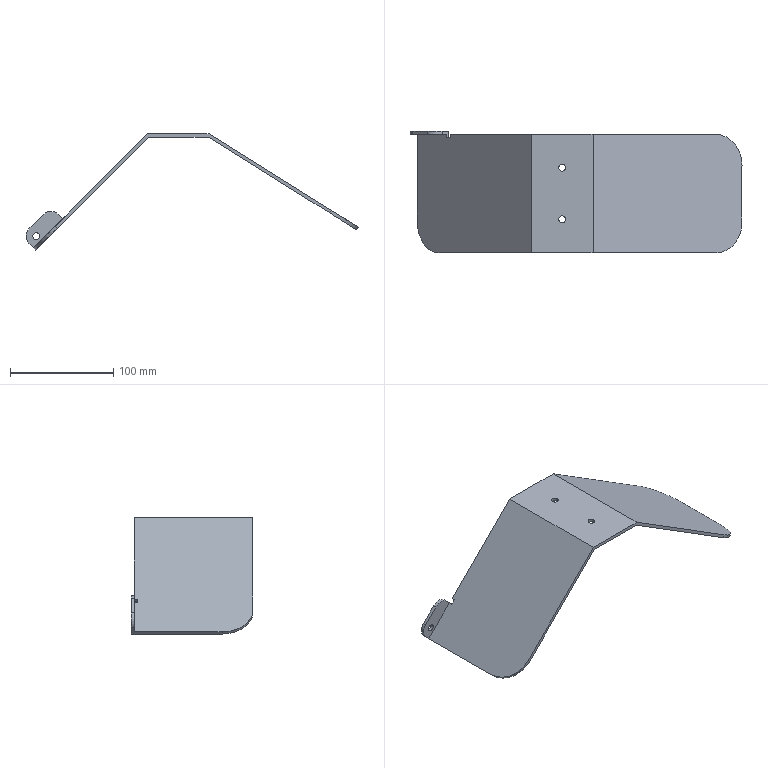Part | SolidWorks | features BaseBody 1 | 1 solid | 27 faces | box 321.953 x 118.25 x 112.625 mm | volume 132694 mm3 | plane 16 | cylinder 11 | commonest cylinder face diameters 6.5 x6 60 x3 20 x2
STEP:
#1=CARTESIAN_POINT('',(617.2,21.,201.536));
#2=VERTEX_POINT('',#1);
#3=CARTESIAN_POINT('',(623.7,21.,201.536));
#4=VERTEX_POINT('',#3);
#5=CARTESIAN_POINT('',(620.45,21.,201.536));
#6=DIRECTION('',(0.,0.,-1.));
#7=DIRECTION('',(1.,0.,0.));
#8=AXIS2_PLACEMENT_3D('',#5,#6,#7);
#9=CIRCLE('',#8,3.25);
#10=EDGE_CURVE('',#2,#4,#9,.T.);
#11=ORIENTED_EDGE('',*,*,#10,.F.);
#12=CARTESIAN_POINT('',(617.2,21.,198.536));
#13=VERTEX_POINT('',#12);
#14=CARTESIAN_POINT('',(617.2,21.,230.536));
#15=DIRECTION('',(0.,0.,-1.));
#16=VECTOR('',#15,1000.);
#17=LINE('',#14,#16);
#18=EDGE_CURVE('',#2,#13,#17,.T.);
#19=ORIENTED_EDGE('',*,*,#18,.T.);
#20=CARTESIAN_POINT('',(623.7,21.,198.536));
#21=VERTEX_POINT('',#20);
#22=CARTESIAN_POINT('',(620.45,21.,198.536));
#23=DIRECTION('',(0.,0.,1.));
#24=DIRECTION('',(1.,0.,0.));
#25=AXIS2_PLACEMENT_3D('',#22,#23,#24);
#26=CIRCLE('',#25,3.25);
#27=EDGE_CURVE('',#21,#13,#26,.T.);
#28=ORIENTED_EDGE('',*,*,#27,.F.);
#29=CARTESIAN_POINT('',(623.7,21.,230.536));
#30=DIRECTION('',(0.,0.,-1.));
#31=VECTOR('',#30,1000.);
#32=LINE('',#29,#31);
#33=EDGE_CURVE('',#4,#21,#32,.T.);
#34=ORIENTED_EDGE('',*,*,#33,.F.);
#35=EDGE_LOOP('',(#11,#19,#28,#34));
#36=FACE_OUTER_BOUND('',#35,.T.);
#37=CARTESIAN_POINT('',(620.45,21.,230.536));
#38=DIRECTION('',(0.,0.,-1.));
#39=DIRECTION('',(1.,0.,0.));
#40=AXIS2_PLACEMENT_3D('',#37,#38,#39);
#41=CYLINDRICAL_SURFACE('',#40,3.25);
#42=ADVANCED_FACE('',(#36),#41,.F.);
#43=CARTESIAN_POINT('',(617.2,-29.,201.536));
#44=VERTEX_POINT('',#43);
#45=CARTESIAN_POINT('',(623.7,-29.,201.536));
#46=VERTEX_POINT('',#45);
#47=CARTESIAN_POINT('',(620.45,-29.,201.536));
#48=DIRECTION('',(0.,0.,-1.));
#49=DIRECTION('',(1.,0.,0.));
#50=AXIS2_PLACEMENT_3D('',#47,#48,#49);
#51=CIRCLE('',#50,3.25);
#52=EDGE_CURVE('',#44,#46,#51,.T.);
#53=ORIENTED_EDGE('',*,*,#52,.F.);
#54=CARTESIAN_POINT('',(617.2,-29.,198.536));
#55=VERTEX_POINT('',#54);
#56=CARTESIAN_POINT('',(617.2,-29.,230.536));
#57=DIRECTION('',(0.,0.,-1.));
#58=VECTOR('',#57,1000.);
#59=LINE('',#56,#58);
#60=EDGE_CURVE('',#44,#55,#59,.T.);
#61=ORIENTED_EDGE('',*,*,#60,.T.);
#62=CARTESIAN_POINT('',(623.7,-29.,198.536));
#63=VERTEX_POINT('',#62);
#64=CARTESIAN_POINT('',(620.45,-29.,198.536));
#65=DIRECTION('',(0.,0.,1.));
#66=DIRECTION('',(1.,0.,0.));
#67=AXIS2_PLACEMENT_3D('',#64,#65,#66);
#68=CIRCLE('',#67,3.25);
#69=EDGE_CURVE('',#63,#55,#68,.T.);
#70=ORIENTED_EDGE('',*,*,#69,.F.);
#71=CARTESIAN_POINT('',(623.7,-29.,230.536));
#72=DIRECTION('',(0.,0.,-1.));
#73=VECTOR('',#72,1000.);
#74=LINE('',#71,#73);
#75=EDGE_CURVE('',#46,#63,#74,.T.);
#76=ORIENTED_EDGE('',*,*,#75,.F.);
#77=EDGE_LOOP('',(#53,#61,#70,#76));
#78=FACE_OUTER_BOUND('',#77,.T.);
#79=CARTESIAN_POINT('',(620.45,-29.,230.536));
#80=DIRECTION('',(0.,0.,-1.));
#81=DIRECTION('',(1.,0.,0.));
#82=AXIS2_PLACEMENT_3D('',#79,#80,#81);
#83=CYLINDRICAL_SURFACE('',#82,3.25);
#84=ADVANCED_FACE('',(#78),#83,.F.);
#85=CARTESIAN_POINT('',(486.098,56.75,102.629));
#86=VERTEX_POINT('',#85);
#87=CARTESIAN_POINT('',(479.623,56.75,102.063));
#88=VERTEX_POINT('',#87);
#89=CARTESIAN_POINT('',(482.86,56.75,102.346));
#90=DIRECTION('',(0.,-1.,0.));
#91=DIRECTION('',(0.,0.,1.));
#92=AXIS2_PLACEMENT_3D('',#89,#90,#91);
#93=CIRCLE('',#92,3.25);
#94=EDGE_CURVE('',#86,#88,#93,.T.);
#95=ORIENTED_EDGE('',*,*,#94,.F.);
#96=CARTESIAN_POINT('',(486.098,53.75,102.629));
#97=VERTEX_POINT('',#96);
#98=CARTESIAN_POINT('',(486.098,94.,102.629));
#99=DIRECTION('',(0.,-1.,0.));
#100=VECTOR('',#99,1000.);
#101=LINE('',#98,#100);
#102=EDGE_CURVE('',#86,#97,#101,.T.);
#103=ORIENTED_EDGE('',*,*,#102,.T.);
#104=CARTESIAN_POINT('',(479.623,53.75,102.063));
#105=VERTEX_POINT('',#104);
#106=CARTESIAN_POINT('',(482.86,53.75,102.346));
#107=DIRECTION('',(0.,1.,0.));
#108=DIRECTION('',(0.,0.,1.));
#109=AXIS2_PLACEMENT_3D('',#106,#107,#108);
#110=CIRCLE('',#109,3.25);
#111=EDGE_CURVE('',#105,#97,#110,.T.);
#112=ORIENTED_EDGE('',*,*,#111,.F.);
#113=CARTESIAN_POINT('',(479.623,94.,102.063));
#114=DIRECTION('',(0.,-1.,0.));
#115=VECTOR('',#114,1000.);
#116=LINE('',#113,#115);
#117=EDGE_CURVE('',#88,#105,#116,.T.);
#118=ORIENTED_EDGE('',*,*,#117,.F.);
#119=EDGE_LOOP('',(#95,#103,#112,#118));
#120=FACE_OUTER_BOUND('',#119,.T.);
#121=CARTESIAN_POINT('',(482.86,94.,102.346));
#122=DIRECTION('',(0.,-1.,0.));
#123=DIRECTION('',(-0.9962,0.,-0.08716));
#124=AXIS2_PLACEMENT_3D('',#121,#122,#123);
#125=CYLINDRICAL_SURFACE('',#124,3.25);
#126=ADVANCED_FACE('',(#120),#125,.F.);
#127=CARTESIAN_POINT('',(511.852,50.5,122.852));
#128=VERTEX_POINT('',#127);
#129=CARTESIAN_POINT('',(511.852,53.5,122.852));
#130=VERTEX_POINT('',#129);
#131=CARTESIAN_POINT('',(511.852,-4.,122.852));
#132=DIRECTION('',(0.,1.,0.));
#133=VECTOR('',#132,1000.);
#134=LINE('',#131,#133);
#135=EDGE_CURVE('',#128,#130,#134,.T.);
#136=ORIENTED_EDGE('',*,*,#135,.T.);
#137=CARTESIAN_POINT('',(513.973,53.5,120.731));
#138=VERTEX_POINT('',#137);
#139=CARTESIAN_POINT('',(511.852,53.5,122.852));
#140=DIRECTION('',(0.7071,0.,-0.7071));
#141=VECTOR('',#140,1000.);
#142=LINE('',#139,#141);
#143=EDGE_CURVE('',#130,#138,#142,.T.);
#144=ORIENTED_EDGE('',*,*,#143,.T.);
#145=CARTESIAN_POINT('',(513.973,50.5,120.731));
#146=VERTEX_POINT('',#145);
#147=CARTESIAN_POINT('',(513.973,-4.,120.731));
#148=DIRECTION('',(0.,1.,0.));
#149=VECTOR('',#148,1000.);
#150=LINE('',#147,#149);
#151=EDGE_CURVE('',#146,#138,#150,.T.);
#152=ORIENTED_EDGE('',*,*,#151,.F.);
#153=CARTESIAN_POINT('',(500.538,50.5,134.166));
#154=DIRECTION('',(0.7071,0.,-0.7071));
#155=VECTOR('',#154,1000.);
#156=LINE('',#153,#155);
#157=EDGE_CURVE('',#128,#146,#156,.T.);
#158=ORIENTED_EDGE('',*,*,#157,.F.);
#159=EDGE_LOOP('',(#136,#144,#152,#158));
#160=FACE_OUTER_BOUND('',#159,.T.);
#161=CARTESIAN_POINT('',(511.852,57.,122.852));
#162=DIRECTION('',(-0.7071,0.,-0.7071));
#163=DIRECTION('',(-0.7071,0.,0.7071));
#164=AXIS2_PLACEMENT_3D('',#161,#162,#163);
#165=PLANE('',#164);
#166=ADVANCED_FACE('',(#160),#165,.T.);
#167=ORIENTED_EDGE('',*,*,#157,.T.);
#168=CARTESIAN_POINT('',(510.437,50.5,117.195));
#169=VERTEX_POINT('',#168);
#170=CARTESIAN_POINT('',(596.251,50.5,203.009));
#171=DIRECTION('',(-0.7071,0.,-0.7071));
#172=VECTOR('',#171,1000.);
#173=LINE('',#170,#172);
#174=EDGE_CURVE('',#146,#169,#173,.T.);
#175=ORIENTED_EDGE('',*,*,#174,.T.);
#176=CARTESIAN_POINT('',(508.316,50.5,119.316));
#177=VERTEX_POINT('',#176);
#178=CARTESIAN_POINT('',(508.316,50.5,119.316));
#179=DIRECTION('',(-0.7071,0.,0.7071));
#180=VECTOR('',#179,1000.);
#181=LINE('',#178,#180);
#182=EDGE_CURVE('',#169,#177,#181,.T.);
#183=ORIENTED_EDGE('',*,*,#182,.T.);
#184=CARTESIAN_POINT('',(594.13,50.5,205.13));
#185=DIRECTION('',(-0.7071,0.,-0.7071));
#186=VECTOR('',#185,1000.);
#187=LINE('',#184,#186);
#188=EDGE_CURVE('',#128,#177,#187,.T.);
#189=ORIENTED_EDGE('',*,*,#188,.F.);
#190=EDGE_LOOP('',(#167,#175,#183,#189));
#191=FACE_OUTER_BOUND('',#190,.T.);
#192=CARTESIAN_POINT('',(500.538,50.5,134.166));
#193=DIRECTION('',(0.,-1.,0.));
#194=DIRECTION('',(0.,0.,-1.));
#195=AXIS2_PLACEMENT_3D('',#192,#193,#194);
#196=PLANE('',#195);
#197=ADVANCED_FACE('',(#191),#196,.F.);
#198=CARTESIAN_POINT('',(767.782,53.5,124.627));
#199=VERTEX_POINT('',#198);
#200=CARTESIAN_POINT('',(793.223,23.5,108.73));
#201=VERTEX_POINT('',#200);
#202=CARTESIAN_POINT('',(767.782,23.5,124.627));
#203=DIRECTION('',(-0.5299,0.,-0.848));
#204=DIRECTION('',(-0.848,0.,0.5299));
#205=AXIS2_PLACEMENT_3D('',#202,#203,#204);
#206=CIRCLE('',#205,30.);
#207=EDGE_CURVE('',#199,#201,#206,.T.);
#208=ORIENTED_EDGE('',*,*,#207,.T.);
#209=CARTESIAN_POINT('',(793.223,-31.5,108.73));
#210=VERTEX_POINT('',#209);
#211=CARTESIAN_POINT('',(793.223,46.,108.73));
#212=DIRECTION('',(0.,-1.,0.));
#213=VECTOR('',#212,1000.);
#214=LINE('',#211,#213);
#215=EDGE_CURVE('',#201,#210,#214,.T.);
#216=ORIENTED_EDGE('',*,*,#215,.T.);
#217=CARTESIAN_POINT('',(767.782,-61.5,124.627));
#218=VERTEX_POINT('',#217);
#219=CARTESIAN_POINT('',(767.782,-31.5,124.627));
#220=DIRECTION('',(-0.5299,0.,-0.848));
#221=DIRECTION('',(0.848,0.,-0.5299));
#222=AXIS2_PLACEMENT_3D('',#219,#220,#221);
#223=CIRCLE('',#222,30.);
#224=EDGE_CURVE('',#210,#218,#223,.T.);
#225=ORIENTED_EDGE('',*,*,#224,.T.);
#226=CARTESIAN_POINT('',(649.504,-61.5,198.536));
#227=VERTEX_POINT('',#226);
#228=CARTESIAN_POINT('',(616.757,-61.5,218.998));
#229=DIRECTION('',(0.848,0.,-0.5299));
#230=VECTOR('',#229,1000.);
#231=LINE('',#228,#230);
#232=EDGE_CURVE('',#227,#218,#231,.T.);
#233=ORIENTED_EDGE('',*,*,#232,.F.);
#234=CARTESIAN_POINT('',(649.504,53.5,198.536));
#235=VERTEX_POINT('',#234);
#236=CARTESIAN_POINT('',(649.504,-4.,198.536));
#237=DIRECTION('',(0.,1.,0.));
#238=VECTOR('',#237,1000.);
#239=LINE('',#236,#238);
#240=EDGE_CURVE('',#227,#235,#239,.T.);
#241=ORIENTED_EDGE('',*,*,#240,.T.);
#242=CARTESIAN_POINT('',(624.235,53.5,214.325));
#243=DIRECTION('',(-0.848,0.,0.5299));
#244=VECTOR('',#243,1000.);
#245=LINE('',#242,#244);
#246=EDGE_CURVE('',#199,#235,#245,.T.);
#247=ORIENTED_EDGE('',*,*,#246,.F.);
#248=EDGE_LOOP('',(#208,#216,#225,#233,#241,#247));
#249=FACE_OUTER_BOUND('',#248,.T.);
#250=CARTESIAN_POINT('',(616.757,-4.,218.998));
#251=DIRECTION('',(-0.5299,0.,-0.848));
#252=DIRECTION('',(-0.848,0.,0.5299));
#253=AXIS2_PLACEMENT_3D('',#250,#251,#252);
#254=PLANE('',#253);
#255=ADVANCED_FACE('',(#249),#254,.T.);
#256=CARTESIAN_POINT('',(769.372,-61.5,127.172));
#257=VERTEX_POINT('',#256);
#258=CARTESIAN_POINT('',(767.782,-61.5,124.627));
#259=DIRECTION('',(0.5299,0.,0.848));
#260=VECTOR('',#259,1000.);
#261=LINE('',#258,#260);
#262=EDGE_CURVE('',#218,#257,#261,.T.);
#263=ORIENTED_EDGE('',*,*,#262,.F.);
#264=ORIENTED_EDGE('',*,*,#224,.F.);
#265=CARTESIAN_POINT('',(794.813,-31.5,111.274));
#266=VERTEX_POINT('',#265);
#267=CARTESIAN_POINT('',(793.223,-31.5,108.73));
#268=DIRECTION('',(0.5299,0.,0.848));
#269=VECTOR('',#268,1000.);
#270=LINE('',#267,#269);
#271=EDGE_CURVE('',#210,#266,#270,.T.);
#272=ORIENTED_EDGE('',*,*,#271,.T.);
#273=CARTESIAN_POINT('',(769.372,-31.5,127.172));
#274=DIRECTION('',(0.5299,0.,0.848));
#275=DIRECTION('',(0.,-1.,0.));
#276=AXIS2_PLACEMENT_3D('',#273,#274,#275);
#277=CIRCLE('',#276,30.);
#278=EDGE_CURVE('',#257,#266,#277,.T.);
#279=ORIENTED_EDGE('',*,*,#278,.F.);
#280=EDGE_LOOP('',(#263,#264,#272,#279));
#281=FACE_OUTER_BOUND('',#280,.T.);
#282=CARTESIAN_POINT('',(769.372,-31.5,127.172));
#283=DIRECTION('',(-0.5299,0.,-0.848));
#284=DIRECTION('',(-0.848,0.,0.5299));
#285=AXIS2_PLACEMENT_3D('',#282,#283,#284);
#286=CYLINDRICAL_SURFACE('',#285,30.);
#287=ADVANCED_FACE('',(#281),#286,.T.);
#288=CARTESIAN_POINT('',(794.813,23.5,111.274));
#289=VERTEX_POINT('',#288);
#290=CARTESIAN_POINT('',(794.813,23.5,111.274));
#291=DIRECTION('',(-0.5299,0.,-0.848));
#292=VECTOR('',#291,1000.);
#293=LINE('',#290,#292);
#294=EDGE_CURVE('',#289,#201,#293,.T.);
#295=ORIENTED_EDGE('',*,*,#294,.T.);
#296=ORIENTED_EDGE('',*,*,#207,.F.);
#297=CARTESIAN_POINT('',(769.372,53.5,127.172));
#298=VERTEX_POINT('',#297);
#299=CARTESIAN_POINT('',(769.372,53.5,127.172));
#300=DIRECTION('',(-0.5299,0.,-0.848));
#301=VECTOR('',#300,1000.);
#302=LINE('',#299,#301);
#303=EDGE_CURVE('',#298,#199,#302,.T.);
#304=ORIENTED_EDGE('',*,*,#303,.F.);
#305=CARTESIAN_POINT('',(769.372,23.5,127.172));
#306=DIRECTION('',(0.5299,0.,0.848));
#307=DIRECTION('',(-0.848,0.,0.5299));
#308=AXIS2_PLACEMENT_3D('',#305,#306,#307);
#309=CIRCLE('',#308,30.);
#310=EDGE_CURVE('',#289,#298,#309,.T.);
#311=ORIENTED_EDGE('',*,*,#310,.F.);
#312=EDGE_LOOP('',(#295,#296,#304,#311));
#313=FACE_OUTER_BOUND('',#312,.T.);
#314=CARTESIAN_POINT('',(769.372,23.5,127.172));
#315=DIRECTION('',(-0.5299,0.,-0.848));
#316=DIRECTION('',(0.848,0.,-0.5299));
#317=AXIS2_PLACEMENT_3D('',#314,#315,#316);
#318=CYLINDRICAL_SURFACE('',#317,30.);
#319=ADVANCED_FACE('',(#313),#318,.T.);
#320=ORIENTED_EDGE('',*,*,#294,.F.);
#321=CARTESIAN_POINT('',(794.813,46.,111.274));
#322=DIRECTION('',(0.,-1.,0.));
#323=VECTOR('',#322,1000.);
#324=LINE('',#321,#323);
#325=EDGE_CURVE('',#289,#266,#324,.T.);
#326=ORIENTED_EDGE('',*,*,#325,.T.);
#327=ORIENTED_EDGE('',*,*,#271,.F.);
#328=ORIENTED_EDGE('',*,*,#215,.F.);
#329=EDGE_LOOP('',(#320,#326,#327,#328));
#330=FACE_OUTER_BOUND('',#329,.T.);
#331=CARTESIAN_POINT('',(794.813,46.,111.274));
#332=DIRECTION('',(-0.848,0.,0.5299));
#333=DIRECTION('',(0.,1.,0.));
#334=AXIS2_PLACEMENT_3D('',#331,#332,#333);
#335=PLANE('',#334);
#336=ADVANCED_FACE('',(#330),#335,.F.);
#337=CARTESIAN_POINT('',(650.364,-61.5,201.536));
#338=VERTEX_POINT('',#337);
#339=CARTESIAN_POINT('',(650.364,53.5,201.536));
#340=VERTEX_POINT('',#339);
#341=CARTESIAN_POINT('',(650.364,-4.,201.536));
#342=DIRECTION('',(0.,1.,0.));
#343=VECTOR('',#342,1000.);
#344=LINE('',#341,#343);
#345=EDGE_CURVE('',#338,#340,#344,.T.);
#346=ORIENTED_EDGE('',*,*,#345,.F.);
#347=CARTESIAN_POINT('',(618.347,-61.5,221.542));
#348=DIRECTION('',(-0.848,0.,0.5299));
#349=VECTOR('',#348,1000.);
#350=LINE('',#347,#349);
#351=EDGE_CURVE('',#257,#338,#350,.T.);
#352=ORIENTED_EDGE('',*,*,#351,.F.);
#353=ORIENTED_EDGE('',*,*,#278,.T.);
#354=ORIENTED_EDGE('',*,*,#325,.F.);
#355=ORIENTED_EDGE('',*,*,#310,.T.);
#356=CARTESIAN_POINT('',(618.347,53.5,221.542));
#357=DIRECTION('',(-0.848,0.,0.5299));
#358=VECTOR('',#357,1000.);
#359=LINE('',#356,#358);
#360=EDGE_CURVE('',#298,#340,#359,.T.);
#361=ORIENTED_EDGE('',*,*,#360,.T.);
#362=EDGE_LOOP('',(#346,#352,#353,#354,#355,#361));
#363=FACE_OUTER_BOUND('',#362,.T.);
#364=CARTESIAN_POINT('',(618.347,-4.,221.542));
#365=DIRECTION('',(-0.5299,0.,-0.848));
#366=DIRECTION('',(-0.848,0.,0.5299));
#367=AXIS2_PLACEMENT_3D('',#364,#365,#366);
#368=PLANE('',#367);
#369=ADVANCED_FACE('',(#363),#368,.F.);
#370=CARTESIAN_POINT('',(482.153,56.75,88.911));
#371=VERTEX_POINT('',#370);
#372=CARTESIAN_POINT('',(475.789,56.75,95.275));
#373=VERTEX_POINT('',#372);
#374=CARTESIAN_POINT('',(480.032,56.75,91.032));
#375=DIRECTION('',(-0.7071,0.,0.7071));
#376=VECTOR('',#375,1000.);
#377=LINE('',#374,#376);
#378=EDGE_CURVE('',#371,#373,#377,.T.);
#379=ORIENTED_EDGE('',*,*,#378,.F.);
#380=CARTESIAN_POINT('',(482.153,-31.5,88.911));
#381=VERTEX_POINT('',#380);
#382=CARTESIAN_POINT('',(482.153,-24.,88.911));
#383=DIRECTION('',(0.,1.,0.));
#384=VECTOR('',#383,1000.);
#385=LINE('',#382,#384);
#386=EDGE_CURVE('',#381,#371,#385,.T.);
#387=ORIENTED_EDGE('',*,*,#386,.F.);
#388=CARTESIAN_POINT('',(480.032,-31.5,91.032));
#389=VERTEX_POINT('',#388);
#390=CARTESIAN_POINT('',(480.032,-31.5,91.032));
#391=DIRECTION('',(0.7071,0.,-0.7071));
#392=VECTOR('',#391,1000.);
#393=LINE('',#390,#392);
#394=EDGE_CURVE('',#389,#381,#393,.T.);
#395=ORIENTED_EDGE('',*,*,#394,.F.);
#396=CARTESIAN_POINT('',(480.032,53.75,91.032));
#397=VERTEX_POINT('',#396);
#398=CARTESIAN_POINT('',(480.032,-24.,91.032));
#399=DIRECTION('',(0.,1.,0.));
#400=VECTOR('',#399,1000.);
#401=LINE('',#398,#400);
#402=EDGE_CURVE('',#389,#397,#401,.T.);
#403=ORIENTED_EDGE('',*,*,#402,.T.);
#404=CARTESIAN_POINT('',(475.789,53.75,95.275));
#405=VERTEX_POINT('',#404);
#406=CARTESIAN_POINT('',(468.718,53.75,102.346));
#407=DIRECTION('',(0.7071,0.,-0.7071));
#408=VECTOR('',#407,1000.);
#409=LINE('',#406,#408);
#410=EDGE_CURVE('',#405,#397,#409,.T.);
#411=ORIENTED_EDGE('',*,*,#410,.F.);
#412=CARTESIAN_POINT('',(475.789,57.,95.275));
#413=DIRECTION('',(0.,-1.,0.));
#414=VECTOR('',#413,1000.);
#415=LINE('',#412,#414);
#416=EDGE_CURVE('',#373,#405,#415,.T.);
#417=ORIENTED_EDGE('',*,*,#416,.F.);
#418=EDGE_LOOP('',(#379,#387,#395,#403,#411,#417));
#419=FACE_OUTER_BOUND('',#418,.T.);
#420=CARTESIAN_POINT('',(480.032,-54.,91.032));
#421=DIRECTION('',(0.7071,0.,0.7071));
#422=DIRECTION('',(0.,-1.,0.));
#423=AXIS2_PLACEMENT_3D('',#420,#421,#422);
#424=PLANE('',#423);
#425=ADVANCED_FACE('',(#419),#424,.F.);
#426=ORIENTED_EDGE('',*,*,#111,.T.);
#427=CARTESIAN_POINT('',(482.86,53.75,102.346));
#428=DIRECTION('',(0.,1.,0.));
#429=DIRECTION('',(0.,0.,1.));
#430=AXIS2_PLACEMENT_3D('',#427,#428,#429);
#431=CIRCLE('',#430,3.25);
#432=EDGE_CURVE('',#97,#105,#431,.T.);
#433=ORIENTED_EDGE('',*,*,#432,.T.);
#434=EDGE_LOOP('',(#426,#433));
#435=FACE_BOUND('',#434,.T.);
#436=ORIENTED_EDGE('',*,*,#410,.T.);
#437=CARTESIAN_POINT('',(508.316,53.75,119.316));
#438=VERTEX_POINT('',#437);
#439=CARTESIAN_POINT('',(594.13,53.75,205.13));
#440=DIRECTION('',(0.7071,0.,0.7071));
#441=VECTOR('',#440,1000.);
#442=LINE('',#439,#441);
#443=EDGE_CURVE('',#397,#438,#442,.T.);
#444=ORIENTED_EDGE('',*,*,#443,.T.);
#445=CARTESIAN_POINT('',(504.073,53.75,123.559));
#446=VERTEX_POINT('',#445);
#447=CARTESIAN_POINT('',(497.002,53.75,130.63));
#448=DIRECTION('',(-0.7071,0.,0.7071));
#449=VECTOR('',#448,1000.);
#450=LINE('',#447,#449);
#451=EDGE_CURVE('',#438,#446,#450,.T.);
#452=ORIENTED_EDGE('',*,*,#451,.T.);
#453=CARTESIAN_POINT('',(489.931,53.75,123.559));
#454=VERTEX_POINT('',#453);
#455=CARTESIAN_POINT('',(497.002,53.75,116.488));
#456=DIRECTION('',(0.,-1.,0.));
#457=DIRECTION('',(0.,0.,1.));
#458=AXIS2_PLACEMENT_3D('',#455,#456,#457);
#459=CIRCLE('',#458,10.);
#460=EDGE_CURVE('',#446,#454,#459,.T.);
#461=ORIENTED_EDGE('',*,*,#460,.T.);
#462=CARTESIAN_POINT('',(475.789,53.75,109.417));
#463=VERTEX_POINT('',#462);
#464=CARTESIAN_POINT('',(582.816,53.75,216.444));
#465=DIRECTION('',(-0.7071,0.,-0.7071));
#466=VECTOR('',#465,1000.);
#467=LINE('',#464,#466);
#468=EDGE_CURVE('',#454,#463,#467,.T.);
#469=ORIENTED_EDGE('',*,*,#468,.T.);
#470=CARTESIAN_POINT('',(482.86,53.75,102.346));
#471=DIRECTION('',(0.,-1.,0.));
#472=DIRECTION('',(0.,0.,1.));
#473=AXIS2_PLACEMENT_3D('',#470,#471,#472);
#474=CIRCLE('',#473,10.);
#475=EDGE_CURVE('',#463,#405,#474,.T.);
#476=ORIENTED_EDGE('',*,*,#475,.T.);
#477=EDGE_LOOP('',(#436,#444,#452,#461,#469,#476));
#478=FACE_OUTER_BOUND('',#477,.T.);
#479=CARTESIAN_POINT('',(468.718,53.75,102.346));
#480=DIRECTION('',(0.,1.,0.));
#481=DIRECTION('',(1.,0.,0.));
#482=AXIS2_PLACEMENT_3D('',#479,#480,#481);
#483=PLANE('',#482);
#484=ADVANCED_FACE('',(#435,#478),#483,.F.);
#485=CARTESIAN_POINT('',(475.789,56.75,109.417));
#486=VERTEX_POINT('',#485);
#487=CARTESIAN_POINT('',(475.789,54.,109.417));
#488=DIRECTION('',(0.,1.,0.));
#489=VECTOR('',#488,1000.);
#490=LINE('',#487,#489);
#491=EDGE_CURVE('',#463,#486,#490,.T.);
#492=ORIENTED_EDGE('',*,*,#491,.F.);
#493=ORIENTED_EDGE('',*,*,#468,.F.);
#494=CARTESIAN_POINT('',(489.931,56.75,123.559));
#495=VERTEX_POINT('',#494);
#496=CARTESIAN_POINT('',(489.931,57.,123.559));
#497=DIRECTION('',(0.,-1.,0.));
#498=VECTOR('',#497,1000.);
#499=LINE('',#496,#498);
#500=EDGE_CURVE('',#495,#454,#499,.T.);
#501=ORIENTED_EDGE('',*,*,#500,.F.);
#502=CARTESIAN_POINT('',(582.816,56.75,216.444));
#503=DIRECTION('',(0.7071,0.,0.7071));
#504=VECTOR('',#503,1000.);
#505=LINE('',#502,#504);
#506=EDGE_CURVE('',#486,#495,#505,.T.);
#507=ORIENTED_EDGE('',*,*,#506,.F.);
#508=EDGE_LOOP('',(#492,#493,#501,#507));
#509=FACE_OUTER_BOUND('',#508,.T.);
#510=CARTESIAN_POINT('',(582.816,-4.,216.444));
#511=DIRECTION('',(-0.7071,0.,0.7071));
#512=DIRECTION('',(0.,1.,0.));
#513=AXIS2_PLACEMENT_3D('',#510,#511,#512);
#514=PLANE('',#513);
#515=ADVANCED_FACE('',(#509),#514,.T.);
#516=ORIENTED_EDGE('',*,*,#451,.F.);
#517=CARTESIAN_POINT('',(508.316,57.,119.316));
#518=DIRECTION('',(0.,-1.,0.));
#519=VECTOR('',#518,1000.);
#520=LINE('',#517,#519);
#521=EDGE_CURVE('',#438,#177,#520,.T.);
#522=ORIENTED_EDGE('',*,*,#521,.T.);
#523=ORIENTED_EDGE('',*,*,#182,.F.);
#524=CARTESIAN_POINT('',(510.437,56.75,117.195));
#525=VERTEX_POINT('',#524);
#526=CARTESIAN_POINT('',(510.437,-4.,117.195));
#527=DIRECTION('',(0.,1.,0.));
#528=VECTOR('',#527,1000.);
#529=LINE('',#526,#528);
#530=EDGE_CURVE('',#169,#525,#529,.T.);
#531=ORIENTED_EDGE('',*,*,#530,.T.);
#532=CARTESIAN_POINT('',(504.073,56.75,123.559));
#533=VERTEX_POINT('',#532);
#534=CARTESIAN_POINT('',(508.316,56.75,119.316));
#535=DIRECTION('',(0.7071,0.,-0.7071));
#536=VECTOR('',#535,1000.);
#537=LINE('',#534,#536);
#538=EDGE_CURVE('',#533,#525,#537,.T.);
#539=ORIENTED_EDGE('',*,*,#538,.F.);
#540=CARTESIAN_POINT('',(504.073,54.,123.559));
#541=DIRECTION('',(0.,1.,0.));
#542=VECTOR('',#541,1000.);
#543=LINE('',#540,#542);
#544=EDGE_CURVE('',#446,#533,#543,.T.);
#545=ORIENTED_EDGE('',*,*,#544,.F.);
#546=EDGE_LOOP('',(#516,#522,#523,#531,#539,#545));
#547=FACE_OUTER_BOUND('',#546,.T.);
#548=CARTESIAN_POINT('',(508.316,57.,119.316));
#549=DIRECTION('',(-0.7071,0.,-0.7071));
#550=DIRECTION('',(-0.7071,0.,0.7071));
#551=AXIS2_PLACEMENT_3D('',#548,#549,#550);
#552=PLANE('',#551);
#553=ADVANCED_FACE('',(#547),#552,.F.);
#554=ORIENTED_EDGE('',*,*,#394,.T.);
#555=CARTESIAN_POINT('',(503.366,-61.5,110.124));
#556=VERTEX_POINT('',#555);
#557=CARTESIAN_POINT('',(503.366,-31.5,110.124));
#558=DIRECTION('',(0.7071,0.,-0.7071));
#559=DIRECTION('',(0.,-1.,0.));
#560=AXIS2_PLACEMENT_3D('',#557,#558,#559);
#561=CIRCLE('',#560,30.);
#562=EDGE_CURVE('',#556,#381,#561,.T.);
#563=ORIENTED_EDGE('',*,*,#562,.F.);
#564=CARTESIAN_POINT('',(501.245,-61.5,112.245));
#565=VERTEX_POINT('',#564);
#566=CARTESIAN_POINT('',(501.245,-61.5,112.245));
#567=DIRECTION('',(0.7071,0.,-0.7071));
#568=VECTOR('',#567,1000.);
#569=LINE('',#566,#568);
#570=EDGE_CURVE('',#565,#556,#569,.T.);
#571=ORIENTED_EDGE('',*,*,#570,.F.);
#572=CARTESIAN_POINT('',(501.245,-31.5,112.245));
#573=DIRECTION('',(-0.7071,0.,0.7071));
#574=DIRECTION('',(-0.7071,0.,-0.7071));
#575=AXIS2_PLACEMENT_3D('',#572,#573,#574);
#576=CIRCLE('',#575,30.);
#577=EDGE_CURVE('',#389,#565,#576,.T.);
#578=ORIENTED_EDGE('',*,*,#577,.F.);
#579=EDGE_LOOP('',(#554,#563,#571,#578));
#580=FACE_OUTER_BOUND('',#579,.T.);
#581=CARTESIAN_POINT('',(501.245,-31.5,112.245));
#582=DIRECTION('',(0.7071,0.,-0.7071));
#583=DIRECTION('',(-0.7071,0.,-0.7071));
#584=AXIS2_PLACEMENT_3D('',#581,#582,#583);
#585=CYLINDRICAL_SURFACE('',#584,30.);
#586=ADVANCED_FACE('',(#580),#585,.T.);
#587=ORIENTED_EDGE('',*,*,#544,.T.);
#588=CARTESIAN_POINT('',(497.002,56.75,116.488));
#589=DIRECTION('',(0.,1.,0.));
#590=DIRECTION('',(0.,0.,1.));
#591=AXIS2_PLACEMENT_3D('',#588,#589,#590);
#592=CIRCLE('',#591,10.);
#593=EDGE_CURVE('',#495,#533,#592,.T.);
#594=ORIENTED_EDGE('',*,*,#593,.F.);
#595=ORIENTED_EDGE('',*,*,#500,.T.);
#596=ORIENTED_EDGE('',*,*,#460,.F.);
#597=EDGE_LOOP('',(#587,#594,#595,#596));
#598=FACE_OUTER_BOUND('',#597,.T.);
#599=CARTESIAN_POINT('',(497.002,-4.,116.488));
#600=DIRECTION('',(0.,-1.,0.));
#601=DIRECTION('',(-0.9962,0.,-0.08716));
#602=AXIS2_PLACEMENT_3D('',#599,#600,#601);
#603=CYLINDRICAL_SURFACE('',#602,10.);
#604=ADVANCED_FACE('',(#598),#603,.T.);
#605=ORIENTED_EDGE('',*,*,#416,.T.);
#606=ORIENTED_EDGE('',*,*,#475,.F.);
#607=ORIENTED_EDGE('',*,*,#491,.T.);
#608=CARTESIAN_POINT('',(482.86,56.75,102.346));
#609=DIRECTION('',(0.,1.,0.));
#610=DIRECTION('',(0.,0.,1.));
#611=AXIS2_PLACEMENT_3D('',#608,#609,#610);
#612=CIRCLE('',#611,10.);
#613=EDGE_CURVE('',#373,#486,#612,.T.);
#614=ORIENTED_EDGE('',*,*,#613,.F.);
#615=EDGE_LOOP('',(#605,#606,#607,#614));
#616=FACE_OUTER_BOUND('',#615,.T.);
#617=CARTESIAN_POINT('',(482.86,-4.,102.346));
#618=DIRECTION('',(0.,1.,0.));
#619=DIRECTION('',(0.9962,0.,0.08716));
#620=AXIS2_PLACEMENT_3D('',#617,#618,#619);
#621=CYLINDRICAL_SURFACE('',#620,10.);
#622=ADVANCED_FACE('',(#616),#621,.T.);
#623=ORIENTED_EDGE('',*,*,#102,.F.);
#624=CARTESIAN_POINT('',(482.86,56.75,102.346));
#625=DIRECTION('',(0.,-1.,0.));
#626=DIRECTION('',(0.,0.,1.));
#627=AXIS2_PLACEMENT_3D('',#624,#625,#626);
#628=CIRCLE('',#627,3.25);
#629=EDGE_CURVE('',#88,#86,#628,.T.);
#630=ORIENTED_EDGE('',*,*,#629,.F.);
#631=ORIENTED_EDGE('',*,*,#117,.T.);
#632=ORIENTED_EDGE('',*,*,#432,.F.);
#633=EDGE_LOOP('',(#623,#630,#631,#632));
#634=FACE_OUTER_BOUND('',#633,.T.);
#635=CARTESIAN_POINT('',(482.86,94.,102.346));
#636=DIRECTION('',(0.,-1.,0.));
#637=DIRECTION('',(-0.9962,0.,-0.08716));
#638=AXIS2_PLACEMENT_3D('',#635,#636,#637);
#639=CYLINDRICAL_SURFACE('',#638,3.25);
#640=ADVANCED_FACE('',(#634),#639,.F.);
#641=ORIENTED_EDGE('',*,*,#135,.F.);
#642=ORIENTED_EDGE('',*,*,#188,.T.);
#643=ORIENTED_EDGE('',*,*,#521,.F.);
#644=ORIENTED_EDGE('',*,*,#443,.F.);
#645=ORIENTED_EDGE('',*,*,#402,.F.);
#646=ORIENTED_EDGE('',*,*,#577,.T.);
#647=CARTESIAN_POINT('',(590.535,-61.5,201.536));
#648=VERTEX_POINT('',#647);
#649=CARTESIAN_POINT('',(618.086,-61.5,229.087));
#650=DIRECTION('',(-0.7071,0.,-0.7071));
#651=VECTOR('',#650,1000.);
#652=LINE('',#649,#651);
#653=EDGE_CURVE('',#648,#565,#652,.T.);
#654=ORIENTED_EDGE('',*,*,#653,.F.);
#655=CARTESIAN_POINT('',(590.535,53.5,201.536));
#656=VERTEX_POINT('',#655);
#657=CARTESIAN_POINT('',(590.535,-4.,201.536));
#658=DIRECTION('',(0.,-1.,0.));
#659=VECTOR('',#658,1000.);
#660=LINE('',#657,#659);
#661=EDGE_CURVE('',#656,#648,#660,.T.);
#662=ORIENTED_EDGE('',*,*,#661,.F.);
#663=CARTESIAN_POINT('',(594.13,53.5,205.13));
#664=DIRECTION('',(-0.7071,0.,-0.7071));
#665=VECTOR('',#664,1000.);
#666=LINE('',#663,#665);
#667=EDGE_CURVE('',#656,#130,#666,.T.);
#668=ORIENTED_EDGE('',*,*,#667,.T.);
#669=EDGE_LOOP('',(#641,#642,#643,#644,#645,#646,#654,#662,#668));
#670=FACE_OUTER_BOUND('',#669,.T.);
#671=CARTESIAN_POINT('',(594.13,-4.,205.13));
#672=DIRECTION('',(0.7071,0.,-0.7071));
#673=DIRECTION('',(0.,-1.,0.));
#674=AXIS2_PLACEMENT_3D('',#671,#672,#673);
#675=PLANE('',#674);
#676=ADVANCED_FACE('',(#670),#675,.F.);
#677=ORIENTED_EDGE('',*,*,#351,.T.);
#678=CARTESIAN_POINT('',(649.374,-61.5,201.536));
#679=DIRECTION('',(1.,0.,0.));
#680=VECTOR('',#679,1000.);
#681=LINE('',#678,#680);
#682=EDGE_CURVE('',#648,#338,#681,.T.);
#683=ORIENTED_EDGE('',*,*,#682,.F.);
#684=ORIENTED_EDGE('',*,*,#653,.T.);
#685=ORIENTED_EDGE('',*,*,#570,.T.);
#686=CARTESIAN_POINT('',(591.778,-61.5,198.536));
#687=VERTEX_POINT('',#686);
#688=CARTESIAN_POINT('',(596.251,-61.5,203.009));
#689=DIRECTION('',(0.7071,0.,0.7071));
#690=VECTOR('',#689,1000.);
#691=LINE('',#688,#690);
#692=EDGE_CURVE('',#556,#687,#691,.T.);
#693=ORIENTED_EDGE('',*,*,#692,.T.);
#694=CARTESIAN_POINT('',(609.504,-61.5,198.536));
#695=DIRECTION('',(-1.,0.,0.));
#696=VECTOR('',#695,1000.);
#697=LINE('',#694,#696);
#698=EDGE_CURVE('',#227,#687,#697,.T.);
#699=ORIENTED_EDGE('',*,*,#698,.F.);
#700=ORIENTED_EDGE('',*,*,#232,.T.);
#701=ORIENTED_EDGE('',*,*,#262,.T.);
#702=EDGE_LOOP('',(#677,#683,#684,#685,#693,#699,#700,#701));
#703=FACE_OUTER_BOUND('',#702,.T.);
#704=CARTESIAN_POINT('',(649.374,-61.5,197.799));
#705=DIRECTION('',(0.,1.,0.));
#706=DIRECTION('',(1.,0.,0.));
#707=AXIS2_PLACEMENT_3D('',#704,#705,#706);
#708=PLANE('',#707);
#709=ADVANCED_FACE('',(#703),#708,.F.);
#710=ORIENTED_EDGE('',*,*,#143,.F.);
#711=ORIENTED_EDGE('',*,*,#667,.F.);
#712=CARTESIAN_POINT('',(609.504,53.5,201.536));
#713=DIRECTION('',(-1.,0.,0.));
#714=VECTOR('',#713,1000.);
#715=LINE('',#712,#714);
#716=EDGE_CURVE('',#340,#656,#715,.T.);
#717=ORIENTED_EDGE('',*,*,#716,.F.);
#718=ORIENTED_EDGE('',*,*,#360,.F.);
#719=ORIENTED_EDGE('',*,*,#303,.T.);
#720=ORIENTED_EDGE('',*,*,#246,.T.);
#721=CARTESIAN_POINT('',(591.778,53.5,198.536));
#722=VERTEX_POINT('',#721);
#723=CARTESIAN_POINT('',(609.122,53.5,198.536));
#724=DIRECTION('',(1.,0.,0.));
#725=VECTOR('',#724,1000.);
#726=LINE('',#723,#725);
#727=EDGE_CURVE('',#722,#235,#726,.T.);
#728=ORIENTED_EDGE('',*,*,#727,.F.);
#729=CARTESIAN_POINT('',(596.251,53.5,203.009));
#730=DIRECTION('',(-0.7071,0.,-0.7071));
#731=VECTOR('',#730,1000.);
#732=LINE('',#729,#731);
#733=EDGE_CURVE('',#722,#138,#732,.T.);
#734=ORIENTED_EDGE('',*,*,#733,.T.);
#735=EDGE_LOOP('',(#710,#711,#717,#718,#719,#720,#728,#734));
#736=FACE_OUTER_BOUND('',#735,.T.);
#737=CARTESIAN_POINT('',(609.122,53.5,190.138));
#738=DIRECTION('',(0.,1.,0.));
#739=DIRECTION('',(1.,0.,0.));
#740=AXIS2_PLACEMENT_3D('',#737,#738,#739);
#741=PLANE('',#740);
#742=ADVANCED_FACE('',(#736),#741,.T.);
#743=CARTESIAN_POINT('',(620.45,-29.,201.536));
#744=DIRECTION('',(0.,0.,-1.));
#745=DIRECTION('',(1.,0.,0.));
#746=AXIS2_PLACEMENT_3D('',#743,#744,#745);
#747=CIRCLE('',#746,3.25);
#748=EDGE_CURVE('',#46,#44,#747,.T.);
#749=ORIENTED_EDGE('',*,*,#748,.T.);
#750=ORIENTED_EDGE('',*,*,#52,.T.);
#751=EDGE_LOOP('',(#749,#750));
#752=FACE_BOUND('',#751,.T.);
#753=CARTESIAN_POINT('',(620.45,21.,201.536));
#754=DIRECTION('',(0.,0.,-1.));
#755=DIRECTION('',(1.,0.,0.));
#756=AXIS2_PLACEMENT_3D('',#753,#754,#755);
#757=CIRCLE('',#756,3.25);
#758=EDGE_CURVE('',#4,#2,#757,.T.);
#759=ORIENTED_EDGE('',*,*,#758,.T.);
#760=ORIENTED_EDGE('',*,*,#10,.T.);
#761=EDGE_LOOP('',(#759,#760));
#762=FACE_BOUND('',#761,.T.);
#763=ORIENTED_EDGE('',*,*,#682,.T.);
#764=ORIENTED_EDGE('',*,*,#345,.T.);
#765=ORIENTED_EDGE('',*,*,#716,.T.);
#766=ORIENTED_EDGE('',*,*,#661,.T.);
#767=EDGE_LOOP('',(#763,#764,#765,#766));
#768=FACE_OUTER_BOUND('',#767,.T.);
#769=CARTESIAN_POINT('',(609.504,-4.,201.536));
#770=DIRECTION('',(0.,0.,1.));
#771=DIRECTION('',(1.,0.,0.));
#772=AXIS2_PLACEMENT_3D('',#769,#770,#771);
#773=PLANE('',#772);
#774=ADVANCED_FACE('',(#752,#762,#768),#773,.T.);
#775=ORIENTED_EDGE('',*,*,#27,.T.);
#776=CARTESIAN_POINT('',(620.45,21.,198.536));
#777=DIRECTION('',(0.,0.,1.));
#778=DIRECTION('',(1.,0.,0.));
#779=AXIS2_PLACEMENT_3D('',#776,#777,#778);
#780=CIRCLE('',#779,3.25);
#781=EDGE_CURVE('',#13,#21,#780,.T.);
#782=ORIENTED_EDGE('',*,*,#781,.T.);
#783=EDGE_LOOP('',(#775,#782));
#784=FACE_BOUND('',#783,.T.);
#785=ORIENTED_EDGE('',*,*,#69,.T.);
#786=CARTESIAN_POINT('',(620.45,-29.,198.536));
#787=DIRECTION('',(0.,0.,1.));
#788=DIRECTION('',(1.,0.,0.));
#789=AXIS2_PLACEMENT_3D('',#786,#787,#788);
#790=CIRCLE('',#789,3.25);
#791=EDGE_CURVE('',#55,#63,#790,.T.);
#792=ORIENTED_EDGE('',*,*,#791,.T.);
#793=EDGE_LOOP('',(#785,#792));
#794=FACE_BOUND('',#793,.T.);
#795=ORIENTED_EDGE('',*,*,#240,.F.);
#796=ORIENTED_EDGE('',*,*,#698,.T.);
#797=CARTESIAN_POINT('',(591.778,-4.,198.536));
#798=DIRECTION('',(0.,1.,0.));
#799=VECTOR('',#798,1000.);
#800=LINE('',#797,#799);
#801=EDGE_CURVE('',#687,#722,#800,.T.);
#802=ORIENTED_EDGE('',*,*,#801,.T.);
#803=ORIENTED_EDGE('',*,*,#727,.T.);
#804=EDGE_LOOP('',(#795,#796,#802,#803));
#805=FACE_OUTER_BOUND('',#804,.T.);
#806=CARTESIAN_POINT('',(609.504,-4.,198.536));
#807=DIRECTION('',(0.,0.,1.));
#808=DIRECTION('',(1.,0.,0.));
#809=AXIS2_PLACEMENT_3D('',#806,#807,#808);
#810=PLANE('',#809);
#811=ADVANCED_FACE('',(#784,#794,#805),#810,.F.);
#812=ORIENTED_EDGE('',*,*,#174,.F.);
#813=ORIENTED_EDGE('',*,*,#151,.T.);
#814=ORIENTED_EDGE('',*,*,#733,.F.);
#815=ORIENTED_EDGE('',*,*,#801,.F.);
#816=ORIENTED_EDGE('',*,*,#692,.F.);
#817=ORIENTED_EDGE('',*,*,#562,.T.);
#818=ORIENTED_EDGE('',*,*,#386,.T.);
#819=CARTESIAN_POINT('',(596.251,56.75,203.009));
#820=DIRECTION('',(-0.7071,0.,-0.7071));
#821=VECTOR('',#820,1000.);
#822=LINE('',#819,#821);
#823=EDGE_CURVE('',#525,#371,#822,.T.);
#824=ORIENTED_EDGE('',*,*,#823,.F.);
#825=ORIENTED_EDGE('',*,*,#530,.F.);
#826=EDGE_LOOP('',(#812,#813,#814,#815,#816,#817,#818,#824,#825));
#827=FACE_OUTER_BOUND('',#826,.T.);
#828=CARTESIAN_POINT('',(596.251,-4.,203.009));
#829=DIRECTION('',(0.7071,0.,-0.7071));
#830=DIRECTION('',(0.,-1.,0.));
#831=AXIS2_PLACEMENT_3D('',#828,#829,#830);
#832=PLANE('',#831);
#833=ADVANCED_FACE('',(#827),#832,.T.);
#834=ORIENTED_EDGE('',*,*,#629,.T.);
#835=ORIENTED_EDGE('',*,*,#94,.T.);
#836=EDGE_LOOP('',(#834,#835));
#837=FACE_BOUND('',#836,.T.);
#838=ORIENTED_EDGE('',*,*,#538,.T.);
#839=ORIENTED_EDGE('',*,*,#823,.T.);
#840=ORIENTED_EDGE('',*,*,#378,.T.);
#841=ORIENTED_EDGE('',*,*,#613,.T.);
#842=ORIENTED_EDGE('',*,*,#506,.T.);
#843=ORIENTED_EDGE('',*,*,#593,.T.);
#844=EDGE_LOOP('',(#838,#839,#840,#841,#842,#843));
#845=FACE_OUTER_BOUND('',#844,.T.);
#846=CARTESIAN_POINT('',(609.122,56.75,190.138));
#847=DIRECTION('',(0.,1.,0.));
#848=DIRECTION('',(1.,0.,0.));
#849=AXIS2_PLACEMENT_3D('',#846,#847,#848);
#850=PLANE('',#849);
#851=ADVANCED_FACE('',(#837,#845),#850,.T.);
#852=ORIENTED_EDGE('',*,*,#60,.F.);
#853=ORIENTED_EDGE('',*,*,#748,.F.);
#854=ORIENTED_EDGE('',*,*,#75,.T.);
#855=ORIENTED_EDGE('',*,*,#791,.F.);
#856=EDGE_LOOP('',(#852,#853,#854,#855));
#857=FACE_OUTER_BOUND('',#856,.T.);
#858=CARTESIAN_POINT('',(620.45,-29.,230.536));
#859=DIRECTION('',(0.,0.,-1.));
#860=DIRECTION('',(1.,0.,0.));
#861=AXIS2_PLACEMENT_3D('',#858,#859,#860);
#862=CYLINDRICAL_SURFACE('',#861,3.25);
#863=ADVANCED_FACE('',(#857),#862,.F.);
#864=ORIENTED_EDGE('',*,*,#18,.F.);
#865=ORIENTED_EDGE('',*,*,#758,.F.);
#866=ORIENTED_EDGE('',*,*,#33,.T.);
#867=ORIENTED_EDGE('',*,*,#781,.F.);
#868=EDGE_LOOP('',(#864,#865,#866,#867));
#869=FACE_OUTER_BOUND('',#868,.T.);
#870=CARTESIAN_POINT('',(620.45,21.,230.536));
#871=DIRECTION('',(0.,0.,-1.));
#872=DIRECTION('',(1.,0.,0.));
#873=AXIS2_PLACEMENT_3D('',#870,#871,#872);
#874=CYLINDRICAL_SURFACE('',#873,3.25);
#875=ADVANCED_FACE('',(#869),#874,.F.);
#876=CLOSED_SHELL('',(#42,#84,#126,#166,#197,#255,#287,#319,#336,#369,#425,#484,#515,#553,#586,#604,#622,#640,#676,#709,#742,#774,#811,#833,#851,#863,#875));
#877=MANIFOLD_SOLID_BREP('',#876);
#878=CARTESIAN_POINT('',(0.,0.,0.));
#879=DIRECTION('',(0.,0.,1.));
#880=DIRECTION('',(1.,0.,0.));
#881=AXIS2_PLACEMENT_3D('',#878,#879,#880);
#882=(LENGTH_UNIT()NAMED_UNIT(*)SI_UNIT(.MILLI.,.METRE.));
#883=UNCERTAINTY_MEASURE_WITH_UNIT(LENGTH_MEASURE(0.00001),#882,'','');
#884=(NAMED_UNIT(*)PLANE_ANGLE_UNIT()SI_UNIT($,.RADIAN.));
#885=(NAMED_UNIT(*)SI_UNIT($,.STERADIAN.)SOLID_ANGLE_UNIT());
#886=(GEOMETRIC_REPRESENTATION_CONTEXT(3)GLOBAL_UNCERTAINTY_ASSIGNED_CONTEXT((#883))GLOBAL_UNIT_ASSIGNED_CONTEXT((#882,#884,#885))REPRESENTATION_CONTEXT('',''));
#887=ADVANCED_BREP_SHAPE_REPRESENTATION('',(#877,#881),#886);